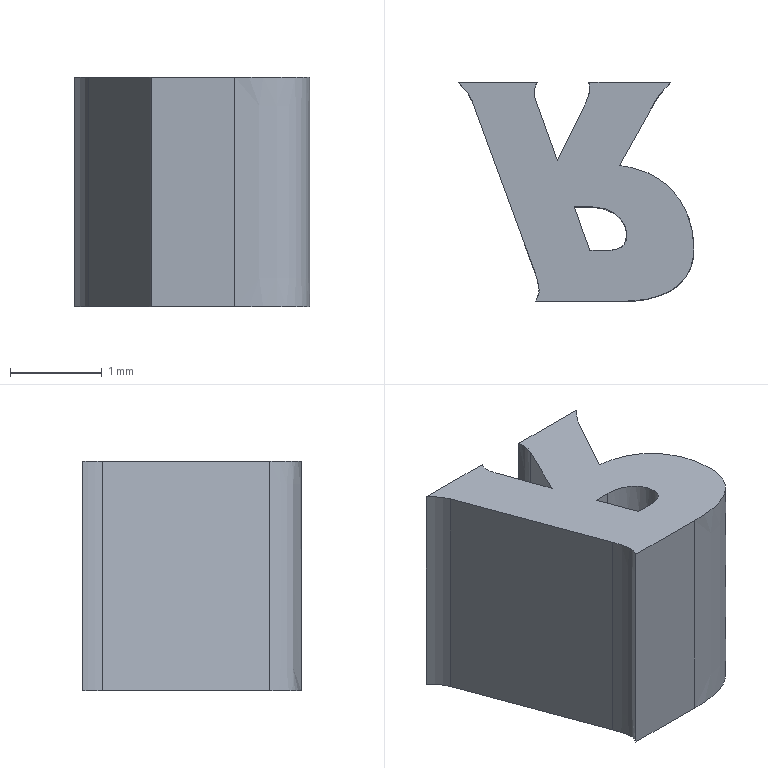Part | STEP file | lll_id1094_x_t | 1 solid | 23 faces | box 2.571 x 2.384 x 2.5 mm | volume 9.133 mm3 | plane 12 | other 6 | cylinder 5 | commonest cylinder face diameters 0.399 x1 1.039 x1 1.183 x1 1.552 x1 2.628 x1
STEP:
#1=CARTESIAN_POINT('',(386.73,-124.408,2.35));
#2=VERTEX_POINT('',#1);
#3=CARTESIAN_POINT('',(386.771,-124.406,2.35));
#4=VERTEX_POINT('',#3);
#5=CARTESIAN_POINT('',(386.726,-123.816,2.35));
#6=DIRECTION('',(0.,0.,1.));
#7=DIRECTION('',(0.,1.,0.));
#8=AXIS2_PLACEMENT_3D('',#5,#6,#7);
#9=CIRCLE('',#8,0.5916);
#10=EDGE_CURVE('',#2,#4,#9,.T.);
#11=ORIENTED_EDGE('',*,*,#10,.T.);
#12=CARTESIAN_POINT('',(386.771,-124.406,-0.15));
#13=VERTEX_POINT('',#12);
#14=CARTESIAN_POINT('',(386.771,-124.406,-0.15));
#15=DIRECTION('',(0.,0.,1.));
#16=VECTOR('',#15,1.);
#17=LINE('',#14,#16);
#18=EDGE_CURVE('',#13,#4,#17,.T.);
#19=ORIENTED_EDGE('',*,*,#18,.F.);
#20=CARTESIAN_POINT('',(386.73,-124.408,-0.15));
#21=VERTEX_POINT('',#20);
#22=CARTESIAN_POINT('',(386.726,-123.816,-0.15));
#23=DIRECTION('',(0.,0.,1.));
#24=DIRECTION('',(-1.,0.,0.));
#25=AXIS2_PLACEMENT_3D('',#22,#23,#24);
#26=CIRCLE('',#25,0.5916);
#27=EDGE_CURVE('',#21,#13,#26,.T.);
#28=ORIENTED_EDGE('',*,*,#27,.F.);
#29=CARTESIAN_POINT('',(386.73,-124.408,-0.15));
#30=DIRECTION('',(0.,0.,1.));
#31=VECTOR('',#30,1.);
#32=LINE('',#29,#31);
#33=EDGE_CURVE('',#21,#2,#32,.T.);
#34=ORIENTED_EDGE('',*,*,#33,.T.);
#35=EDGE_LOOP('',(#11,#19,#28,#34));
#36=FACE_OUTER_BOUND('',#35,.T.);
#37=CARTESIAN_POINT('',(386.726,-123.816,-0.15));
#38=DIRECTION('',(0.,0.,1.));
#39=DIRECTION('',(1.,0.,0.));
#40=AXIS2_PLACEMENT_3D('',#37,#38,#39);
#41=CYLINDRICAL_SURFACE('',#40,0.5916);
#42=ADVANCED_FACE('',(#36),#41,.F.);
#43=CARTESIAN_POINT('',(386.916,-124.343,2.35));
#44=VERTEX_POINT('',#43);
#45=CARTESIAN_POINT('',(386.771,-124.406,2.35));
#46=CARTESIAN_POINT('',(386.794,-124.405,2.35));
#47=CARTESIAN_POINT('',(386.816,-124.4,2.35));
#48=CARTESIAN_POINT('',(386.853,-124.389,2.35));
#49=CARTESIAN_POINT('',(386.867,-124.382,2.35));
#50=CARTESIAN_POINT('',(386.894,-124.366,2.35));
#51=CARTESIAN_POINT('',(386.906,-124.355,2.35));
#52=CARTESIAN_POINT('',(386.916,-124.343,2.35));
#53=(BOUNDED_CURVE()B_SPLINE_CURVE(3,(#45,#46,#47,#48,#49,#50,#51,#52),.UNSPECIFIED.,.F.,.F.)B_SPLINE_CURVE_WITH_KNOTS((4,2,2,4),(0.,0.418,0.7101,1.),.UNSPECIFIED.)CURVE()GEOMETRIC_REPRESENTATION_ITEM()RATIONAL_B_SPLINE_CURVE((0.5001,0.4979,0.4979,0.4976,0.4976,0.495,0.495,0.5001))REPRESENTATION_ITEM(''));
#54=EDGE_CURVE('',#4,#44,#53,.T.);
#55=ORIENTED_EDGE('',*,*,#54,.T.);
#56=CARTESIAN_POINT('',(386.916,-124.343,-0.15));
#57=VERTEX_POINT('',#56);
#58=CARTESIAN_POINT('',(386.916,-124.343,-0.15));
#59=DIRECTION('',(0.,0.,1.));
#60=VECTOR('',#59,1.);
#61=LINE('',#58,#60);
#62=EDGE_CURVE('',#57,#44,#61,.T.);
#63=ORIENTED_EDGE('',*,*,#62,.F.);
#64=CARTESIAN_POINT('',(386.771,-124.406,-0.15));
#65=CARTESIAN_POINT('',(386.794,-124.405,-0.15));
#66=CARTESIAN_POINT('',(386.816,-124.4,-0.15));
#67=CARTESIAN_POINT('',(386.853,-124.389,-0.15));
#68=CARTESIAN_POINT('',(386.867,-124.382,-0.15));
#69=CARTESIAN_POINT('',(386.894,-124.366,-0.15));
#70=CARTESIAN_POINT('',(386.906,-124.355,-0.15));
#71=CARTESIAN_POINT('',(386.916,-124.343,-0.15));
#72=(BOUNDED_CURVE()B_SPLINE_CURVE(3,(#64,#65,#66,#67,#68,#69,#70,#71),.UNSPECIFIED.,.F.,.F.)B_SPLINE_CURVE_WITH_KNOTS((4,2,2,4),(0.,0.418,0.7101,1.),.UNSPECIFIED.)CURVE()GEOMETRIC_REPRESENTATION_ITEM()RATIONAL_B_SPLINE_CURVE((0.5001,0.4979,0.4979,0.4976,0.4976,0.495,0.495,0.5001))REPRESENTATION_ITEM(''));
#73=EDGE_CURVE('',#13,#57,#72,.T.);
#74=ORIENTED_EDGE('',*,*,#73,.F.);
#75=ORIENTED_EDGE('',*,*,#18,.T.);
#76=EDGE_LOOP('',(#55,#63,#74,#75));
#77=FACE_OUTER_BOUND('',#76,.T.);
#78=CARTESIAN_POINT('',(386.771,-124.406,-0.15));
#79=CARTESIAN_POINT('',(386.794,-124.405,-0.15));
#80=CARTESIAN_POINT('',(386.816,-124.4,-0.15));
#81=CARTESIAN_POINT('',(386.853,-124.389,-0.15));
#82=CARTESIAN_POINT('',(386.867,-124.382,-0.15));
#83=CARTESIAN_POINT('',(386.894,-124.366,-0.15));
#84=CARTESIAN_POINT('',(386.906,-124.355,-0.15));
#85=CARTESIAN_POINT('',(386.916,-124.343,-0.15));
#86=(BOUNDED_CURVE()B_SPLINE_CURVE(3,(#78,#79,#80,#81,#82,#83,#84,#85),.UNSPECIFIED.,.F.,.F.)B_SPLINE_CURVE_WITH_KNOTS((4,2,2,4),(0.,0.418,0.7101,1.),.UNSPECIFIED.)CURVE()GEOMETRIC_REPRESENTATION_ITEM()RATIONAL_B_SPLINE_CURVE((0.5001,0.4979,0.4979,0.4976,0.4976,0.495,0.495,0.5001))REPRESENTATION_ITEM(''));
#87=DIRECTION('',(0.,0.,1.));
#88=VECTOR('',#87,1.);
#89=SURFACE_OF_LINEAR_EXTRUSION('',#86,#88);
#90=ADVANCED_FACE('',(#77),#89,.F.);
#91=CARTESIAN_POINT('',(386.549,-123.934,2.35));
#92=VERTEX_POINT('',#91);
#93=CARTESIAN_POINT('',(386.916,-124.343,2.35));
#94=CARTESIAN_POINT('',(386.927,-124.328,2.35));
#95=CARTESIAN_POINT('',(386.935,-124.312,2.35));
#96=CARTESIAN_POINT('',(386.942,-124.278,2.35));
#97=CARTESIAN_POINT('',(386.944,-124.263,2.35));
#98=CARTESIAN_POINT('',(386.943,-124.185,2.35));
#99=CARTESIAN_POINT('',(386.922,-124.126,2.35));
#100=CARTESIAN_POINT('',(386.859,-124.046,2.35));
#101=CARTESIAN_POINT('',(386.828,-124.018,2.35));
#102=CARTESIAN_POINT('',(386.759,-123.976,2.35));
#103=CARTESIAN_POINT('',(386.722,-123.96,2.35));
#104=CARTESIAN_POINT('',(386.656,-123.944,2.35));
#105=CARTESIAN_POINT('',(386.629,-123.939,2.35));
#106=CARTESIAN_POINT('',(386.589,-123.936,2.35));
#107=CARTESIAN_POINT('',(386.576,-123.935,2.35));
#108=CARTESIAN_POINT('',(386.558,-123.934,2.35));
#109=CARTESIAN_POINT('',(386.553,-123.934,2.35));
#110=CARTESIAN_POINT('',(386.549,-123.934,2.35));
#111=(BOUNDED_CURVE()B_SPLINE_CURVE(3,(#93,#94,#95,#96,#97,#98,#99,#100,#101,#102,#103,#104,#105,#106,#107,#108,#109,#110),.UNSPECIFIED.,.F.,.F.)B_SPLINE_CURVE_WITH_KNOTS((4,2,2,2,2,2,2,2,4),(0.,0.08567,0.1598,0.4394,0.6214,0.8013,0.9206,0.9801,1.),.UNSPECIFIED.)CURVE()GEOMETRIC_REPRESENTATION_ITEM()RATIONAL_B_SPLINE_CURVE((0.5001,0.4929,0.4929,0.4976,0.4976,0.4831,0.4831,0.4948,0.4948,0.4962,0.4962,0.4991,0.4991,0.5,0.5,0.5001,0.5001,0.5001))REPRESENTATION_ITEM(''));
#112=EDGE_CURVE('',#44,#92,#111,.T.);
#113=ORIENTED_EDGE('',*,*,#112,.T.);
#114=CARTESIAN_POINT('',(386.549,-123.934,-0.15));
#115=VERTEX_POINT('',#114);
#116=CARTESIAN_POINT('',(386.549,-123.934,-0.15));
#117=DIRECTION('',(0.,0.,1.));
#118=VECTOR('',#117,1.);
#119=LINE('',#116,#118);
#120=EDGE_CURVE('',#115,#92,#119,.T.);
#121=ORIENTED_EDGE('',*,*,#120,.F.);
#122=CARTESIAN_POINT('',(386.916,-124.343,-0.15));
#123=CARTESIAN_POINT('',(386.927,-124.328,-0.15));
#124=CARTESIAN_POINT('',(386.935,-124.312,-0.15));
#125=CARTESIAN_POINT('',(386.942,-124.278,-0.15));
#126=CARTESIAN_POINT('',(386.944,-124.263,-0.15));
#127=CARTESIAN_POINT('',(386.943,-124.185,-0.15));
#128=CARTESIAN_POINT('',(386.922,-124.126,-0.15));
#129=CARTESIAN_POINT('',(386.859,-124.046,-0.15));
#130=CARTESIAN_POINT('',(386.828,-124.018,-0.15));
#131=CARTESIAN_POINT('',(386.759,-123.976,-0.15));
#132=CARTESIAN_POINT('',(386.722,-123.96,-0.15));
#133=CARTESIAN_POINT('',(386.656,-123.944,-0.15));
#134=CARTESIAN_POINT('',(386.629,-123.939,-0.15));
#135=CARTESIAN_POINT('',(386.589,-123.936,-0.15));
#136=CARTESIAN_POINT('',(386.576,-123.935,-0.15));
#137=CARTESIAN_POINT('',(386.558,-123.934,-0.15));
#138=CARTESIAN_POINT('',(386.553,-123.934,-0.15));
#139=CARTESIAN_POINT('',(386.549,-123.934,-0.15));
#140=(BOUNDED_CURVE()B_SPLINE_CURVE(3,(#122,#123,#124,#125,#126,#127,#128,#129,#130,#131,#132,#133,#134,#135,#136,#137,#138,#139),.UNSPECIFIED.,.F.,.F.)B_SPLINE_CURVE_WITH_KNOTS((4,2,2,2,2,2,2,2,4),(0.,0.08567,0.1598,0.4394,0.6214,0.8013,0.9206,0.9801,1.),.UNSPECIFIED.)CURVE()GEOMETRIC_REPRESENTATION_ITEM()RATIONAL_B_SPLINE_CURVE((0.5001,0.4929,0.4929,0.4976,0.4976,0.4831,0.4831,0.4948,0.4948,0.4962,0.4962,0.4991,0.4991,0.5,0.5,0.5001,0.5001,0.5001))REPRESENTATION_ITEM(''));
#141=EDGE_CURVE('',#57,#115,#140,.T.);
#142=ORIENTED_EDGE('',*,*,#141,.F.);
#143=ORIENTED_EDGE('',*,*,#62,.T.);
#144=EDGE_LOOP('',(#113,#121,#142,#143));
#145=FACE_OUTER_BOUND('',#144,.T.);
#146=CARTESIAN_POINT('',(386.916,-124.343,-0.15));
#147=CARTESIAN_POINT('',(386.927,-124.328,-0.15));
#148=CARTESIAN_POINT('',(386.935,-124.312,-0.15));
#149=CARTESIAN_POINT('',(386.942,-124.278,-0.15));
#150=CARTESIAN_POINT('',(386.944,-124.263,-0.15));
#151=CARTESIAN_POINT('',(386.943,-124.185,-0.15));
#152=CARTESIAN_POINT('',(386.922,-124.126,-0.15));
#153=CARTESIAN_POINT('',(386.859,-124.046,-0.15));
#154=CARTESIAN_POINT('',(386.828,-124.018,-0.15));
#155=CARTESIAN_POINT('',(386.759,-123.976,-0.15));
#156=CARTESIAN_POINT('',(386.722,-123.96,-0.15));
#157=CARTESIAN_POINT('',(386.656,-123.944,-0.15));
#158=CARTESIAN_POINT('',(386.629,-123.939,-0.15));
#159=CARTESIAN_POINT('',(386.589,-123.936,-0.15));
#160=CARTESIAN_POINT('',(386.576,-123.935,-0.15));
#161=CARTESIAN_POINT('',(386.558,-123.934,-0.15));
#162=CARTESIAN_POINT('',(386.553,-123.934,-0.15));
#163=CARTESIAN_POINT('',(386.549,-123.934,-0.15));
#164=(BOUNDED_CURVE()B_SPLINE_CURVE(3,(#146,#147,#148,#149,#150,#151,#152,#153,#154,#155,#156,#157,#158,#159,#160,#161,#162,#163),.UNSPECIFIED.,.F.,.F.)B_SPLINE_CURVE_WITH_KNOTS((4,2,2,2,2,2,2,2,4),(0.,0.08567,0.1598,0.4394,0.6214,0.8013,0.9206,0.9801,1.),.UNSPECIFIED.)CURVE()GEOMETRIC_REPRESENTATION_ITEM()RATIONAL_B_SPLINE_CURVE((0.5001,0.4929,0.4929,0.4976,0.4976,0.4831,0.4831,0.4948,0.4948,0.4962,0.4962,0.4991,0.4991,0.5,0.5,0.5001,0.5001,0.5001))REPRESENTATION_ITEM(''));
#165=DIRECTION('',(0.,0.,1.));
#166=VECTOR('',#165,1.);
#167=SURFACE_OF_LINEAR_EXTRUSION('',#164,#166);
#168=ADVANCED_FACE('',(#145),#167,.F.);
#169=CARTESIAN_POINT('',(386.37,-123.934,2.35));
#170=VERTEX_POINT('',#169);
#171=CARTESIAN_POINT('',(386.549,-123.934,2.35));
#172=DIRECTION('',(-1.,0.,0.));
#173=VECTOR('',#172,1.);
#174=LINE('',#171,#173);
#175=EDGE_CURVE('',#92,#170,#174,.T.);
#176=ORIENTED_EDGE('',*,*,#175,.T.);
#177=CARTESIAN_POINT('',(386.37,-123.934,-0.15));
#178=VERTEX_POINT('',#177);
#179=CARTESIAN_POINT('',(386.37,-123.934,-0.15));
#180=DIRECTION('',(0.,0.,1.));
#181=VECTOR('',#180,1.);
#182=LINE('',#179,#181);
#183=EDGE_CURVE('',#178,#170,#182,.T.);
#184=ORIENTED_EDGE('',*,*,#183,.F.);
#185=CARTESIAN_POINT('',(386.549,-123.934,-0.15));
#186=DIRECTION('',(-1.,0.,0.));
#187=VECTOR('',#186,1.);
#188=LINE('',#185,#187);
#189=EDGE_CURVE('',#115,#178,#188,.T.);
#190=ORIENTED_EDGE('',*,*,#189,.F.);
#191=ORIENTED_EDGE('',*,*,#120,.T.);
#192=EDGE_LOOP('',(#176,#184,#190,#191));
#193=FACE_OUTER_BOUND('',#192,.T.);
#194=CARTESIAN_POINT('',(386.549,-123.934,-0.15));
#195=DIRECTION('',(0.,1.,0.));
#196=DIRECTION('',(0.,0.,1.));
#197=AXIS2_PLACEMENT_3D('',#194,#195,#196);
#198=PLANE('',#197);
#199=ADVANCED_FACE('',(#193),#198,.F.);
#200=CARTESIAN_POINT('',(386.543,-124.408,2.35));
#201=VERTEX_POINT('',#200);
#202=CARTESIAN_POINT('',(386.37,-123.934,2.35));
#203=DIRECTION('',(0.3422,-0.9396,0.));
#204=VECTOR('',#203,1.);
#205=LINE('',#202,#204);
#206=EDGE_CURVE('',#170,#201,#205,.T.);
#207=ORIENTED_EDGE('',*,*,#206,.T.);
#208=CARTESIAN_POINT('',(386.543,-124.408,-0.15));
#209=VERTEX_POINT('',#208);
#210=CARTESIAN_POINT('',(386.543,-124.408,-0.15));
#211=DIRECTION('',(0.,0.,1.));
#212=VECTOR('',#211,1.);
#213=LINE('',#210,#212);
#214=EDGE_CURVE('',#209,#201,#213,.T.);
#215=ORIENTED_EDGE('',*,*,#214,.F.);
#216=CARTESIAN_POINT('',(386.37,-123.934,-0.15));
#217=DIRECTION('',(0.3422,-0.9396,0.));
#218=VECTOR('',#217,1.);
#219=LINE('',#216,#218);
#220=EDGE_CURVE('',#178,#209,#219,.T.);
#221=ORIENTED_EDGE('',*,*,#220,.F.);
#222=ORIENTED_EDGE('',*,*,#183,.T.);
#223=EDGE_LOOP('',(#207,#215,#221,#222));
#224=FACE_OUTER_BOUND('',#223,.T.);
#225=CARTESIAN_POINT('',(386.37,-123.934,-0.15));
#226=DIRECTION('',(-0.9396,-0.3422,0.));
#227=DIRECTION('',(-0.3422,0.9396,0.));
#228=AXIS2_PLACEMENT_3D('',#225,#226,#227);
#229=PLANE('',#228);
#230=ADVANCED_FACE('',(#224),#229,.F.);
#231=CARTESIAN_POINT('',(387.422,-122.581,2.35));
#232=VERTEX_POINT('',#231);
#233=CARTESIAN_POINT('',(387.25,-122.793,2.35));
#234=VERTEX_POINT('',#233);
#235=CARTESIAN_POINT('',(387.925,-123.174,2.35));
#236=DIRECTION('',(0.,0.,1.));
#237=DIRECTION('',(-1.,0.,0.));
#238=AXIS2_PLACEMENT_3D('',#235,#236,#237);
#239=CIRCLE('',#238,0.7758);
#240=EDGE_CURVE('',#232,#234,#239,.T.);
#241=ORIENTED_EDGE('',*,*,#240,.T.);
#242=CARTESIAN_POINT('',(387.25,-122.793,-0.15));
#243=VERTEX_POINT('',#242);
#244=CARTESIAN_POINT('',(387.25,-122.793,-0.15));
#245=DIRECTION('',(0.,0.,1.));
#246=VECTOR('',#245,1.);
#247=LINE('',#244,#246);
#248=EDGE_CURVE('',#243,#234,#247,.T.);
#249=ORIENTED_EDGE('',*,*,#248,.F.);
#250=CARTESIAN_POINT('',(387.422,-122.581,-0.15));
#251=VERTEX_POINT('',#250);
#252=CARTESIAN_POINT('',(387.925,-123.174,-0.15));
#253=DIRECTION('',(0.,0.,1.));
#254=DIRECTION('',(-1.,0.,0.));
#255=AXIS2_PLACEMENT_3D('',#252,#253,#254);
#256=CIRCLE('',#255,0.7758);
#257=EDGE_CURVE('',#251,#243,#256,.T.);
#258=ORIENTED_EDGE('',*,*,#257,.F.);
#259=CARTESIAN_POINT('',(387.429,-122.578,-0.15));
#260=DIRECTION('',(0.,0.,1.));
#261=VECTOR('',#260,1.);
#262=LINE('',#259,#261);
#263=EDGE_CURVE('',#251,#232,#262,.T.);
#264=ORIENTED_EDGE('',*,*,#263,.T.);
#265=EDGE_LOOP('',(#241,#249,#258,#264));
#266=FACE_OUTER_BOUND('',#265,.T.);
#267=CARTESIAN_POINT('',(387.925,-123.174,-0.15));
#268=DIRECTION('',(0.,0.,1.));
#269=DIRECTION('',(1.,0.,0.));
#270=AXIS2_PLACEMENT_3D('',#267,#268,#269);
#271=CYLINDRICAL_SURFACE('',#270,0.7758);
#272=ADVANCED_FACE('',(#266),#271,.F.);
#273=CARTESIAN_POINT('',(386.864,-123.485,2.35));
#274=VERTEX_POINT('',#273);
#275=CARTESIAN_POINT('',(387.25,-122.793,2.35));
#276=DIRECTION('',(-0.4865,-0.8737,0.));
#277=VECTOR('',#276,1.);
#278=LINE('',#275,#277);
#279=EDGE_CURVE('',#234,#274,#278,.T.);
#280=ORIENTED_EDGE('',*,*,#279,.T.);
#281=CARTESIAN_POINT('',(386.864,-123.485,-0.15));
#282=VERTEX_POINT('',#281);
#283=CARTESIAN_POINT('',(386.864,-123.485,-0.15));
#284=DIRECTION('',(0.,0.,1.));
#285=VECTOR('',#284,1.);
#286=LINE('',#283,#285);
#287=EDGE_CURVE('',#282,#274,#286,.T.);
#288=ORIENTED_EDGE('',*,*,#287,.F.);
#289=CARTESIAN_POINT('',(387.25,-122.793,-0.15));
#290=DIRECTION('',(-0.4865,-0.8737,0.));
#291=VECTOR('',#290,1.);
#292=LINE('',#289,#291);
#293=EDGE_CURVE('',#243,#282,#292,.T.);
#294=ORIENTED_EDGE('',*,*,#293,.F.);
#295=ORIENTED_EDGE('',*,*,#248,.T.);
#296=EDGE_LOOP('',(#280,#288,#294,#295));
#297=FACE_OUTER_BOUND('',#296,.T.);
#298=CARTESIAN_POINT('',(387.25,-122.793,-0.15));
#299=DIRECTION('',(-0.8737,0.4865,0.));
#300=DIRECTION('',(0.4865,0.8737,0.));
#301=AXIS2_PLACEMENT_3D('',#298,#299,#300);
#302=PLANE('',#301);
#303=ADVANCED_FACE('',(#297),#302,.F.);
#304=CARTESIAN_POINT('',(387.016,-123.513,2.35));
#305=VERTEX_POINT('',#304);
#306=CARTESIAN_POINT('',(386.706,-124.79,2.35));
#307=DIRECTION('',(0.,0.,-1.));
#308=DIRECTION('',(0.,-1.,0.));
#309=AXIS2_PLACEMENT_3D('',#306,#307,#308);
#310=CIRCLE('',#309,1.314);
#311=EDGE_CURVE('',#274,#305,#310,.T.);
#312=ORIENTED_EDGE('',*,*,#311,.T.);
#313=CARTESIAN_POINT('',(387.016,-123.513,-0.15));
#314=VERTEX_POINT('',#313);
#315=CARTESIAN_POINT('',(387.016,-123.513,-0.15));
#316=DIRECTION('',(0.,0.,1.));
#317=VECTOR('',#316,1.);
#318=LINE('',#315,#317);
#319=EDGE_CURVE('',#314,#305,#318,.T.);
#320=ORIENTED_EDGE('',*,*,#319,.F.);
#321=CARTESIAN_POINT('',(386.706,-124.79,-0.15));
#322=DIRECTION('',(0.,0.,-1.));
#323=DIRECTION('',(1.,0.,0.));
#324=AXIS2_PLACEMENT_3D('',#321,#322,#323);
#325=CIRCLE('',#324,1.314);
#326=EDGE_CURVE('',#282,#314,#325,.T.);
#327=ORIENTED_EDGE('',*,*,#326,.F.);
#328=ORIENTED_EDGE('',*,*,#287,.T.);
#329=EDGE_LOOP('',(#312,#320,#327,#328));
#330=FACE_OUTER_BOUND('',#329,.T.);
#331=CARTESIAN_POINT('',(386.706,-124.79,-0.15));
#332=DIRECTION('',(0.,0.,1.));
#333=DIRECTION('',(1.,0.,0.));
#334=AXIS2_PLACEMENT_3D('',#331,#332,#333);
#335=CYLINDRICAL_SURFACE('',#334,1.314);
#336=ADVANCED_FACE('',(#330),#335,.T.);
#337=CARTESIAN_POINT('',(386.856,-124.962,2.35));
#338=VERTEX_POINT('',#337);
#339=CARTESIAN_POINT('',(387.016,-123.513,2.35));
#340=CARTESIAN_POINT('',(387.307,-123.577,2.35));
#341=CARTESIAN_POINT('',(387.527,-123.776,2.35));
#342=CARTESIAN_POINT('',(387.656,-124.17,2.35));
#343=CARTESIAN_POINT('',(387.674,-124.285,2.35));
#344=CARTESIAN_POINT('',(387.673,-124.447,2.35));
#345=CARTESIAN_POINT('',(387.667,-124.492,2.35));
#346=CARTESIAN_POINT('',(387.628,-124.658,2.35));
#347=CARTESIAN_POINT('',(387.555,-124.761,2.35));
#348=CARTESIAN_POINT('',(387.406,-124.858,2.35));
#349=CARTESIAN_POINT('',(387.359,-124.88,2.35));
#350=CARTESIAN_POINT('',(387.25,-124.918,2.35));
#351=CARTESIAN_POINT('',(387.188,-124.934,2.35));
#352=CARTESIAN_POINT('',(387.061,-124.954,2.35));
#353=CARTESIAN_POINT('',(386.997,-124.96,2.35));
#354=CARTESIAN_POINT('',(386.907,-124.962,2.35));
#355=CARTESIAN_POINT('',(386.881,-124.962,2.35));
#356=CARTESIAN_POINT('',(386.856,-124.962,2.35));
#357=(BOUNDED_CURVE()B_SPLINE_CURVE(3,(#339,#340,#341,#342,#343,#344,#345,#346,#347,#348,#349,#350,#351,#352,#353,#354,#355,#356),.UNSPECIFIED.,.F.,.F.)B_SPLINE_CURVE_WITH_KNOTS((4,2,2,2,2,2,2,2,4),(0.,0.3873,0.5378,0.596,0.7502,0.8132,0.891,0.969,1.),.UNSPECIFIED.)CURVE()GEOMETRIC_REPRESENTATION_ITEM()RATIONAL_B_SPLINE_CURVE((0.5004,0.4564,0.4564,0.496,0.496,0.4986,0.4986,0.4762,0.4762,0.498,0.498,0.499,0.499,0.4997,0.4997,0.5004,0.5004,0.5004))REPRESENTATION_ITEM(''));
#358=EDGE_CURVE('',#305,#338,#357,.T.);
#359=ORIENTED_EDGE('',*,*,#358,.T.);
#360=CARTESIAN_POINT('',(386.856,-124.962,-0.15));
#361=VERTEX_POINT('',#360);
#362=CARTESIAN_POINT('',(386.856,-124.962,-0.15));
#363=DIRECTION('',(0.,0.,1.));
#364=VECTOR('',#363,1.);
#365=LINE('',#362,#364);
#366=EDGE_CURVE('',#361,#338,#365,.T.);
#367=ORIENTED_EDGE('',*,*,#366,.F.);
#368=CARTESIAN_POINT('',(387.016,-123.513,-0.15));
#369=CARTESIAN_POINT('',(387.307,-123.577,-0.15));
#370=CARTESIAN_POINT('',(387.527,-123.776,-0.15));
#371=CARTESIAN_POINT('',(387.656,-124.17,-0.15));
#372=CARTESIAN_POINT('',(387.674,-124.285,-0.15));
#373=CARTESIAN_POINT('',(387.673,-124.447,-0.15));
#374=CARTESIAN_POINT('',(387.667,-124.492,-0.15));
#375=CARTESIAN_POINT('',(387.628,-124.658,-0.15));
#376=CARTESIAN_POINT('',(387.555,-124.761,-0.15));
#377=CARTESIAN_POINT('',(387.406,-124.858,-0.15));
#378=CARTESIAN_POINT('',(387.359,-124.88,-0.15));
#379=CARTESIAN_POINT('',(387.25,-124.918,-0.15));
#380=CARTESIAN_POINT('',(387.188,-124.934,-0.15));
#381=CARTESIAN_POINT('',(387.061,-124.954,-0.15));
#382=CARTESIAN_POINT('',(386.997,-124.96,-0.15));
#383=CARTESIAN_POINT('',(386.907,-124.962,-0.15));
#384=CARTESIAN_POINT('',(386.881,-124.962,-0.15));
#385=CARTESIAN_POINT('',(386.856,-124.962,-0.15));
#386=(BOUNDED_CURVE()B_SPLINE_CURVE(3,(#368,#369,#370,#371,#372,#373,#374,#375,#376,#377,#378,#379,#380,#381,#382,#383,#384,#385),.UNSPECIFIED.,.F.,.F.)B_SPLINE_CURVE_WITH_KNOTS((4,2,2,2,2,2,2,2,4),(0.,0.3873,0.5378,0.596,0.7502,0.8132,0.891,0.969,1.),.UNSPECIFIED.)CURVE()GEOMETRIC_REPRESENTATION_ITEM()RATIONAL_B_SPLINE_CURVE((0.5004,0.4564,0.4564,0.496,0.496,0.4986,0.4986,0.4762,0.4762,0.498,0.498,0.499,0.499,0.4997,0.4997,0.5004,0.5004,0.5004))REPRESENTATION_ITEM(''));
#387=EDGE_CURVE('',#314,#361,#386,.T.);
#388=ORIENTED_EDGE('',*,*,#387,.F.);
#389=ORIENTED_EDGE('',*,*,#319,.T.);
#390=EDGE_LOOP('',(#359,#367,#388,#389));
#391=FACE_OUTER_BOUND('',#390,.T.);
#392=CARTESIAN_POINT('',(387.016,-123.513,-0.15));
#393=CARTESIAN_POINT('',(387.307,-123.577,-0.15));
#394=CARTESIAN_POINT('',(387.527,-123.776,-0.15));
#395=CARTESIAN_POINT('',(387.656,-124.17,-0.15));
#396=CARTESIAN_POINT('',(387.674,-124.285,-0.15));
#397=CARTESIAN_POINT('',(387.673,-124.447,-0.15));
#398=CARTESIAN_POINT('',(387.667,-124.492,-0.15));
#399=CARTESIAN_POINT('',(387.628,-124.658,-0.15));
#400=CARTESIAN_POINT('',(387.555,-124.761,-0.15));
#401=CARTESIAN_POINT('',(387.406,-124.858,-0.15));
#402=CARTESIAN_POINT('',(387.359,-124.88,-0.15));
#403=CARTESIAN_POINT('',(387.25,-124.918,-0.15));
#404=CARTESIAN_POINT('',(387.188,-124.934,-0.15));
#405=CARTESIAN_POINT('',(387.061,-124.954,-0.15));
#406=CARTESIAN_POINT('',(386.997,-124.96,-0.15));
#407=CARTESIAN_POINT('',(386.907,-124.962,-0.15));
#408=CARTESIAN_POINT('',(386.881,-124.962,-0.15));
#409=CARTESIAN_POINT('',(386.856,-124.962,-0.15));
#410=(BOUNDED_CURVE()B_SPLINE_CURVE(3,(#392,#393,#394,#395,#396,#397,#398,#399,#400,#401,#402,#403,#404,#405,#406,#407,#408,#409),.UNSPECIFIED.,.F.,.F.)B_SPLINE_CURVE_WITH_KNOTS((4,2,2,2,2,2,2,2,4),(0.,0.3873,0.5378,0.596,0.7502,0.8132,0.891,0.969,1.),.UNSPECIFIED.)CURVE()GEOMETRIC_REPRESENTATION_ITEM()RATIONAL_B_SPLINE_CURVE((0.5004,0.4564,0.4564,0.496,0.496,0.4986,0.4986,0.4762,0.4762,0.498,0.498,0.499,0.499,0.4997,0.4997,0.5004,0.5004,0.5004))REPRESENTATION_ITEM(''));
#411=DIRECTION('',(0.,0.,1.));
#412=VECTOR('',#411,1.);
#413=SURFACE_OF_LINEAR_EXTRUSION('',#410,#412);
#414=ADVANCED_FACE('',(#391),#413,.F.);
#415=CARTESIAN_POINT('',(385.951,-124.959,2.35));
#416=VERTEX_POINT('',#415);
#417=CARTESIAN_POINT('',(386.856,-124.962,2.35));
#418=DIRECTION('',(-1.,0.,0.));
#419=VECTOR('',#418,1.);
#420=LINE('',#417,#419);
#421=EDGE_CURVE('',#338,#416,#420,.T.);
#422=ORIENTED_EDGE('',*,*,#421,.T.);
#423=CARTESIAN_POINT('',(385.951,-124.959,-0.15));
#424=VERTEX_POINT('',#423);
#425=CARTESIAN_POINT('',(385.946,-124.962,-0.15));
#426=DIRECTION('',(0.,0.,1.));
#427=VECTOR('',#426,1.);
#428=LINE('',#425,#427);
#429=EDGE_CURVE('',#424,#416,#428,.T.);
#430=ORIENTED_EDGE('',*,*,#429,.F.);
#431=CARTESIAN_POINT('',(386.856,-124.962,-0.15));
#432=DIRECTION('',(-1.,0.,0.));
#433=VECTOR('',#432,1.);
#434=LINE('',#431,#433);
#435=EDGE_CURVE('',#361,#424,#434,.T.);
#436=ORIENTED_EDGE('',*,*,#435,.F.);
#437=ORIENTED_EDGE('',*,*,#366,.T.);
#438=EDGE_LOOP('',(#422,#430,#436,#437));
#439=FACE_OUTER_BOUND('',#438,.T.);
#440=CARTESIAN_POINT('',(386.856,-124.962,-0.15));
#441=DIRECTION('',(0.,1.,0.));
#442=DIRECTION('',(0.,0.,1.));
#443=AXIS2_PLACEMENT_3D('',#440,#441,#442);
#444=PLANE('',#443);
#445=ADVANCED_FACE('',(#439),#444,.F.);
#446=CARTESIAN_POINT('',(385.934,-124.618,2.35));
#447=VERTEX_POINT('',#446);
#448=CARTESIAN_POINT('',(385.951,-124.956,2.35));
#449=CARTESIAN_POINT('',(385.953,-124.954,2.35));
#450=CARTESIAN_POINT('',(385.956,-124.951,2.35));
#451=CARTESIAN_POINT('',(385.975,-124.925,2.35));
#452=CARTESIAN_POINT('',(385.985,-124.899,2.35));
#453=CARTESIAN_POINT('',(385.99,-124.858,2.35));
#454=CARTESIAN_POINT('',(385.991,-124.845,2.35));
#455=CARTESIAN_POINT('',(385.989,-124.821,2.35));
#456=CARTESIAN_POINT('',(385.988,-124.81,2.35));
#457=CARTESIAN_POINT('',(385.984,-124.789,2.35));
#458=CARTESIAN_POINT('',(385.982,-124.778,2.35));
#459=CARTESIAN_POINT('',(385.977,-124.756,2.35));
#460=CARTESIAN_POINT('',(385.974,-124.745,2.35));
#461=CARTESIAN_POINT('',(385.964,-124.71,2.35));
#462=CARTESIAN_POINT('',(385.957,-124.685,2.35));
#463=CARTESIAN_POINT('',(385.944,-124.646,2.35));
#464=CARTESIAN_POINT('',(385.939,-124.632,2.35));
#465=CARTESIAN_POINT('',(385.934,-124.618,2.35));
#466=(BOUNDED_CURVE()B_SPLINE_CURVE(3,(#448,#449,#450,#451,#452,#453,#454,#455,#456,#457,#458,#459,#460,#461,#462,#463,#464,#465),.UNSPECIFIED.,.F.,.F.)B_SPLINE_CURVE_WITH_KNOTS((4,2,2,2,2,2,2,2,4),(0.,0.03213,0.269,0.3783,0.4714,0.5647,0.6581,0.8757,1.),.UNSPECIFIED.)CURVE()GEOMETRIC_REPRESENTATION_ITEM()RATIONAL_B_SPLINE_CURVE((0.5001,0.5,0.5,0.4887,0.4887,0.4987,0.4987,0.4996,0.4996,0.4998,0.4998,0.5,0.5,0.5,0.5,0.5,0.5,0.5001))REPRESENTATION_ITEM(''));
#467=EDGE_CURVE('',#416,#447,#466,.T.);
#468=ORIENTED_EDGE('',*,*,#467,.T.);
#469=CARTESIAN_POINT('',(385.934,-124.618,-0.15));
#470=VERTEX_POINT('',#469);
#471=CARTESIAN_POINT('',(385.934,-124.618,-0.15));
#472=DIRECTION('',(0.,0.,1.));
#473=VECTOR('',#472,1.);
#474=LINE('',#471,#473);
#475=EDGE_CURVE('',#470,#447,#474,.T.);
#476=ORIENTED_EDGE('',*,*,#475,.F.);
#477=CARTESIAN_POINT('',(385.949,-124.959,-0.15));
#478=CARTESIAN_POINT('',(385.949,-124.958,-0.15));
#479=CARTESIAN_POINT('',(385.95,-124.957,-0.15));
#480=CARTESIAN_POINT('',(385.953,-124.954,-0.15));
#481=CARTESIAN_POINT('',(385.956,-124.951,-0.15));
#482=CARTESIAN_POINT('',(385.975,-124.925,-0.15));
#483=CARTESIAN_POINT('',(385.985,-124.899,-0.15));
#484=CARTESIAN_POINT('',(385.99,-124.858,-0.15));
#485=CARTESIAN_POINT('',(385.991,-124.845,-0.15));
#486=CARTESIAN_POINT('',(385.989,-124.821,-0.15));
#487=CARTESIAN_POINT('',(385.988,-124.81,-0.15));
#488=CARTESIAN_POINT('',(385.984,-124.789,-0.15));
#489=CARTESIAN_POINT('',(385.982,-124.778,-0.15));
#490=CARTESIAN_POINT('',(385.977,-124.756,-0.15));
#491=CARTESIAN_POINT('',(385.974,-124.745,-0.15));
#492=CARTESIAN_POINT('',(385.964,-124.71,-0.15));
#493=CARTESIAN_POINT('',(385.957,-124.685,-0.15));
#494=CARTESIAN_POINT('',(385.944,-124.646,-0.15));
#495=CARTESIAN_POINT('',(385.939,-124.632,-0.15));
#496=CARTESIAN_POINT('',(385.934,-124.618,-0.15));
#497=(BOUNDED_CURVE()B_SPLINE_CURVE(3,(#477,#478,#479,#480,#481,#482,#483,#484,#485,#486,#487,#488,#489,#490,#491,#492,#493,#494,#495,#496),.UNSPECIFIED.,.F.,.F.)B_SPLINE_CURVE_WITH_KNOTS((4,2,2,2,2,2,2,2,2,4),(0.,0.009901,0.04172,0.2762,0.3844,0.4766,0.569,0.6615,0.8769,1.),.UNSPECIFIED.)CURVE()GEOMETRIC_REPRESENTATION_ITEM()RATIONAL_B_SPLINE_CURVE((0.5001,0.5001,0.5001,0.5,0.5,0.4887,0.4887,0.4987,0.4987,0.4996,0.4996,0.4998,0.4998,0.5,0.5,0.5,0.5,0.5,0.5,0.5001))REPRESENTATION_ITEM(''));
#498=EDGE_CURVE('',#424,#470,#497,.T.);
#499=ORIENTED_EDGE('',*,*,#498,.F.);
#500=ORIENTED_EDGE('',*,*,#429,.T.);
#501=EDGE_LOOP('',(#468,#476,#499,#500));
#502=FACE_OUTER_BOUND('',#501,.T.);
#503=CARTESIAN_POINT('',(385.946,-124.962,-0.15));
#504=CARTESIAN_POINT('',(385.947,-124.961,-0.15));
#505=CARTESIAN_POINT('',(385.948,-124.96,-0.15));
#506=CARTESIAN_POINT('',(385.949,-124.958,-0.15));
#507=CARTESIAN_POINT('',(385.95,-124.957,-0.15));
#508=CARTESIAN_POINT('',(385.953,-124.954,-0.15));
#509=CARTESIAN_POINT('',(385.956,-124.951,-0.15));
#510=CARTESIAN_POINT('',(385.975,-124.925,-0.15));
#511=CARTESIAN_POINT('',(385.985,-124.899,-0.15));
#512=CARTESIAN_POINT('',(385.99,-124.858,-0.15));
#513=CARTESIAN_POINT('',(385.991,-124.845,-0.15));
#514=CARTESIAN_POINT('',(385.989,-124.821,-0.15));
#515=CARTESIAN_POINT('',(385.988,-124.81,-0.15));
#516=CARTESIAN_POINT('',(385.984,-124.789,-0.15));
#517=CARTESIAN_POINT('',(385.982,-124.778,-0.15));
#518=CARTESIAN_POINT('',(385.977,-124.756,-0.15));
#519=CARTESIAN_POINT('',(385.974,-124.745,-0.15));
#520=CARTESIAN_POINT('',(385.964,-124.71,-0.15));
#521=CARTESIAN_POINT('',(385.957,-124.685,-0.15));
#522=CARTESIAN_POINT('',(385.944,-124.646,-0.15));
#523=CARTESIAN_POINT('',(385.939,-124.632,-0.15));
#524=CARTESIAN_POINT('',(385.934,-124.618,-0.15));
#525=(BOUNDED_CURVE()B_SPLINE_CURVE(3,(#503,#504,#505,#506,#507,#508,#509,#510,#511,#512,#513,#514,#515,#516,#517,#518,#519,#520,#521,#522,#523,#524),.UNSPECIFIED.,.F.,.F.)B_SPLINE_CURVE_WITH_KNOTS((4,2,2,2,2,2,2,2,2,2,4),(0.,0.01012,0.01992,0.05142,0.2835,0.3906,0.4819,0.5734,0.665,0.8781,1.),.UNSPECIFIED.)CURVE()GEOMETRIC_REPRESENTATION_ITEM()RATIONAL_B_SPLINE_CURVE((0.5001,0.5001,0.5001,0.5001,0.5001,0.5,0.5,0.4887,0.4887,0.4987,0.4987,0.4996,0.4996,0.4998,0.4998,0.5,0.5,0.5,0.5,0.5,0.5,0.5001))REPRESENTATION_ITEM(''));
#526=DIRECTION('',(0.,0.,1.));
#527=VECTOR('',#526,1.);
#528=SURFACE_OF_LINEAR_EXTRUSION('',#525,#527);
#529=ADVANCED_FACE('',(#502),#528,.F.);
#530=CARTESIAN_POINT('',(385.265,-122.793,2.35));
#531=VERTEX_POINT('',#530);
#532=CARTESIAN_POINT('',(385.934,-124.618,2.35));
#533=DIRECTION('',(-0.3441,0.9389,0.));
#534=VECTOR('',#533,1.);
#535=LINE('',#532,#534);
#536=EDGE_CURVE('',#447,#531,#535,.T.);
#537=ORIENTED_EDGE('',*,*,#536,.T.);
#538=CARTESIAN_POINT('',(385.265,-122.793,-0.15));
#539=VERTEX_POINT('',#538);
#540=CARTESIAN_POINT('',(385.265,-122.793,-0.15));
#541=DIRECTION('',(0.,0.,1.));
#542=VECTOR('',#541,1.);
#543=LINE('',#540,#542);
#544=EDGE_CURVE('',#539,#531,#543,.T.);
#545=ORIENTED_EDGE('',*,*,#544,.F.);
#546=CARTESIAN_POINT('',(385.934,-124.618,-0.15));
#547=DIRECTION('',(-0.3441,0.9389,0.));
#548=VECTOR('',#547,1.);
#549=LINE('',#546,#548);
#550=EDGE_CURVE('',#470,#539,#549,.T.);
#551=ORIENTED_EDGE('',*,*,#550,.F.);
#552=ORIENTED_EDGE('',*,*,#475,.T.);
#553=EDGE_LOOP('',(#537,#545,#551,#552));
#554=FACE_OUTER_BOUND('',#553,.T.);
#555=CARTESIAN_POINT('',(385.934,-124.618,-0.15));
#556=DIRECTION('',(0.9389,0.3441,0.));
#557=DIRECTION('',(0.3441,-0.9389,0.));
#558=AXIS2_PLACEMENT_3D('',#555,#556,#557);
#559=PLANE('',#558);
#560=ADVANCED_FACE('',(#554),#559,.F.);
#561=CARTESIAN_POINT('',(385.108,-122.58,2.35));
#562=VERTEX_POINT('',#561);
#563=CARTESIAN_POINT('',(384.783,-122.988,2.35));
#564=DIRECTION('',(0.,0.,1.));
#565=DIRECTION('',(-1.,0.,0.));
#566=AXIS2_PLACEMENT_3D('',#563,#564,#565);
#567=CIRCLE('',#566,0.5196);
#568=EDGE_CURVE('',#531,#562,#567,.T.);
#569=ORIENTED_EDGE('',*,*,#568,.T.);
#570=CARTESIAN_POINT('',(385.108,-122.58,-0.15));
#571=VERTEX_POINT('',#570);
#572=CARTESIAN_POINT('',(385.102,-122.578,-0.15));
#573=DIRECTION('',(0.,0.,1.));
#574=VECTOR('',#573,1.);
#575=LINE('',#572,#574);
#576=EDGE_CURVE('',#571,#562,#575,.T.);
#577=ORIENTED_EDGE('',*,*,#576,.F.);
#578=CARTESIAN_POINT('',(384.783,-122.988,-0.15));
#579=DIRECTION('',(0.,0.,1.));
#580=DIRECTION('',(-1.,0.,0.));
#581=AXIS2_PLACEMENT_3D('',#578,#579,#580);
#582=CIRCLE('',#581,0.5196);
#583=EDGE_CURVE('',#539,#571,#582,.T.);
#584=ORIENTED_EDGE('',*,*,#583,.F.);
#585=ORIENTED_EDGE('',*,*,#544,.T.);
#586=EDGE_LOOP('',(#569,#577,#584,#585));
#587=FACE_OUTER_BOUND('',#586,.T.);
#588=CARTESIAN_POINT('',(384.783,-122.988,-0.15));
#589=DIRECTION('',(0.,0.,1.));
#590=DIRECTION('',(1.,0.,0.));
#591=AXIS2_PLACEMENT_3D('',#588,#589,#590);
#592=CYLINDRICAL_SURFACE('',#591,0.5196);
#593=ADVANCED_FACE('',(#587),#592,.F.);
#594=CARTESIAN_POINT('',(385.968,-122.58,2.35));
#595=VERTEX_POINT('',#594);
#596=CARTESIAN_POINT('',(385.108,-122.578,2.35));
#597=DIRECTION('',(1.,0.,0.));
#598=VECTOR('',#597,1.);
#599=LINE('',#596,#598);
#600=EDGE_CURVE('',#562,#595,#599,.T.);
#601=ORIENTED_EDGE('',*,*,#600,.T.);
#602=CARTESIAN_POINT('',(385.968,-122.58,-0.15));
#603=VERTEX_POINT('',#602);
#604=CARTESIAN_POINT('',(385.972,-122.578,-0.15));
#605=DIRECTION('',(0.,0.,1.));
#606=VECTOR('',#605,1.);
#607=LINE('',#604,#606);
#608=EDGE_CURVE('',#603,#595,#607,.T.);
#609=ORIENTED_EDGE('',*,*,#608,.F.);
#610=CARTESIAN_POINT('',(385.108,-122.578,-0.15));
#611=DIRECTION('',(1.,0.,0.));
#612=VECTOR('',#611,1.);
#613=LINE('',#610,#612);
#614=EDGE_CURVE('',#571,#603,#613,.T.);
#615=ORIENTED_EDGE('',*,*,#614,.F.);
#616=ORIENTED_EDGE('',*,*,#576,.T.);
#617=EDGE_LOOP('',(#601,#609,#615,#616));
#618=FACE_OUTER_BOUND('',#617,.T.);
#619=CARTESIAN_POINT('',(385.108,-122.578,-0.15));
#620=DIRECTION('',(0.,-1.,0.));
#621=DIRECTION('',(0.,0.,-1.));
#622=AXIS2_PLACEMENT_3D('',#619,#620,#621);
#623=PLANE('',#622);
#624=ADVANCED_FACE('',(#618),#623,.F.);
#625=CARTESIAN_POINT('',(385.948,-122.621,2.35));
#626=VERTEX_POINT('',#625);
#627=CARTESIAN_POINT('',(385.969,-122.583,2.35));
#628=CARTESIAN_POINT('',(385.96,-122.595,2.35));
#629=CARTESIAN_POINT('',(385.953,-122.608,2.35));
#630=CARTESIAN_POINT('',(385.948,-122.621,2.35));
#631=(BOUNDED_CURVE()B_SPLINE_CURVE(3,(#627,#628,#629,#630),.UNSPECIFIED.,.F.,.F.)B_SPLINE_CURVE_WITH_KNOTS((4,4),(0.,1.),.UNSPECIFIED.)CURVE()GEOMETRIC_REPRESENTATION_ITEM()RATIONAL_B_SPLINE_CURVE((0.5015,0.4995,0.4995,0.5015))REPRESENTATION_ITEM(''));
#632=EDGE_CURVE('',#595,#626,#631,.T.);
#633=ORIENTED_EDGE('',*,*,#632,.T.);
#634=CARTESIAN_POINT('',(385.948,-122.621,-0.15));
#635=VERTEX_POINT('',#634);
#636=CARTESIAN_POINT('',(385.948,-122.621,-0.15));
#637=DIRECTION('',(0.,0.,1.));
#638=VECTOR('',#637,1.);
#639=LINE('',#636,#638);
#640=EDGE_CURVE('',#635,#626,#639,.T.);
#641=ORIENTED_EDGE('',*,*,#640,.F.);
#642=CARTESIAN_POINT('',(385.969,-122.583,-0.15));
#643=CARTESIAN_POINT('',(385.96,-122.595,-0.15));
#644=CARTESIAN_POINT('',(385.953,-122.608,-0.15));
#645=CARTESIAN_POINT('',(385.948,-122.621,-0.15));
#646=(BOUNDED_CURVE()B_SPLINE_CURVE(3,(#642,#643,#644,#645),.UNSPECIFIED.,.F.,.F.)B_SPLINE_CURVE_WITH_KNOTS((4,4),(0.,1.),.UNSPECIFIED.)CURVE()GEOMETRIC_REPRESENTATION_ITEM()RATIONAL_B_SPLINE_CURVE((0.5015,0.4995,0.4995,0.5015))REPRESENTATION_ITEM(''));
#647=EDGE_CURVE('',#603,#635,#646,.T.);
#648=ORIENTED_EDGE('',*,*,#647,.F.);
#649=ORIENTED_EDGE('',*,*,#608,.T.);
#650=EDGE_LOOP('',(#633,#641,#648,#649));
#651=FACE_OUTER_BOUND('',#650,.T.);
#652=CARTESIAN_POINT('',(386.133,-122.696,-0.15));
#653=DIRECTION('',(0.,0.,1.));
#654=DIRECTION('',(1.,0.,0.));
#655=AXIS2_PLACEMENT_3D('',#652,#653,#654);
#656=CYLINDRICAL_SURFACE('',#655,0.1996);
#657=ADVANCED_FACE('',(#651),#656,.F.);
#658=CARTESIAN_POINT('',(385.958,-122.789,2.35));
#659=VERTEX_POINT('',#658);
#660=CARTESIAN_POINT('',(385.948,-122.621,2.35));
#661=CARTESIAN_POINT('',(385.942,-122.637,2.35));
#662=CARTESIAN_POINT('',(385.938,-122.654,2.35));
#663=CARTESIAN_POINT('',(385.937,-122.677,2.35));
#664=CARTESIAN_POINT('',(385.936,-122.684,2.35));
#665=CARTESIAN_POINT('',(385.937,-122.702,2.35));
#666=CARTESIAN_POINT('',(385.938,-122.713,2.35));
#667=CARTESIAN_POINT('',(385.942,-122.735,2.35));
#668=CARTESIAN_POINT('',(385.944,-122.746,2.35));
#669=CARTESIAN_POINT('',(385.95,-122.768,2.35));
#670=CARTESIAN_POINT('',(385.954,-122.779,2.35));
#671=CARTESIAN_POINT('',(385.958,-122.789,2.35));
#672=(BOUNDED_CURVE()B_SPLINE_CURVE(3,(#660,#661,#662,#663,#664,#665,#666,#667,#668,#669,#670,#671),.UNSPECIFIED.,.F.,.F.)B_SPLINE_CURVE_WITH_KNOTS((4,2,2,2,2,4),(0.,0.2962,0.4138,0.6091,0.8048,1.),.UNSPECIFIED.)CURVE()GEOMETRIC_REPRESENTATION_ITEM()RATIONAL_B_SPLINE_CURVE((0.5015,0.4975,0.4975,0.5011,0.5011,0.5008,0.5008,0.5011,0.5011,0.5013,0.5013,0.5015))REPRESENTATION_ITEM(''));
#673=EDGE_CURVE('',#626,#659,#672,.T.);
#674=ORIENTED_EDGE('',*,*,#673,.T.);
#675=CARTESIAN_POINT('',(385.958,-122.789,-0.15));
#676=VERTEX_POINT('',#675);
#677=CARTESIAN_POINT('',(385.958,-122.789,-0.15));
#678=DIRECTION('',(0.,0.,1.));
#679=VECTOR('',#678,1.);
#680=LINE('',#677,#679);
#681=EDGE_CURVE('',#676,#659,#680,.T.);
#682=ORIENTED_EDGE('',*,*,#681,.F.);
#683=CARTESIAN_POINT('',(385.948,-122.621,-0.15));
#684=CARTESIAN_POINT('',(385.942,-122.637,-0.15));
#685=CARTESIAN_POINT('',(385.938,-122.654,-0.15));
#686=CARTESIAN_POINT('',(385.937,-122.677,-0.15));
#687=CARTESIAN_POINT('',(385.936,-122.684,-0.15));
#688=CARTESIAN_POINT('',(385.937,-122.702,-0.15));
#689=CARTESIAN_POINT('',(385.938,-122.713,-0.15));
#690=CARTESIAN_POINT('',(385.942,-122.735,-0.15));
#691=CARTESIAN_POINT('',(385.944,-122.746,-0.15));
#692=CARTESIAN_POINT('',(385.95,-122.768,-0.15));
#693=CARTESIAN_POINT('',(385.954,-122.779,-0.15));
#694=CARTESIAN_POINT('',(385.958,-122.789,-0.15));
#695=(BOUNDED_CURVE()B_SPLINE_CURVE(3,(#683,#684,#685,#686,#687,#688,#689,#690,#691,#692,#693,#694),.UNSPECIFIED.,.F.,.F.)B_SPLINE_CURVE_WITH_KNOTS((4,2,2,2,2,4),(0.,0.2962,0.4138,0.6091,0.8048,1.),.UNSPECIFIED.)CURVE()GEOMETRIC_REPRESENTATION_ITEM()RATIONAL_B_SPLINE_CURVE((0.5015,0.4975,0.4975,0.5011,0.5011,0.5008,0.5008,0.5011,0.5011,0.5013,0.5013,0.5015))REPRESENTATION_ITEM(''));
#696=EDGE_CURVE('',#635,#676,#695,.T.);
#697=ORIENTED_EDGE('',*,*,#696,.F.);
#698=ORIENTED_EDGE('',*,*,#640,.T.);
#699=EDGE_LOOP('',(#674,#682,#697,#698));
#700=FACE_OUTER_BOUND('',#699,.T.);
#701=CARTESIAN_POINT('',(385.948,-122.621,-0.15));
#702=CARTESIAN_POINT('',(385.942,-122.637,-0.15));
#703=CARTESIAN_POINT('',(385.938,-122.654,-0.15));
#704=CARTESIAN_POINT('',(385.937,-122.677,-0.15));
#705=CARTESIAN_POINT('',(385.936,-122.684,-0.15));
#706=CARTESIAN_POINT('',(385.937,-122.702,-0.15));
#707=CARTESIAN_POINT('',(385.938,-122.713,-0.15));
#708=CARTESIAN_POINT('',(385.942,-122.735,-0.15));
#709=CARTESIAN_POINT('',(385.944,-122.746,-0.15));
#710=CARTESIAN_POINT('',(385.95,-122.768,-0.15));
#711=CARTESIAN_POINT('',(385.954,-122.779,-0.15));
#712=CARTESIAN_POINT('',(385.958,-122.789,-0.15));
#713=(BOUNDED_CURVE()B_SPLINE_CURVE(3,(#701,#702,#703,#704,#705,#706,#707,#708,#709,#710,#711,#712),.UNSPECIFIED.,.F.,.F.)B_SPLINE_CURVE_WITH_KNOTS((4,2,2,2,2,4),(0.,0.2962,0.4138,0.6091,0.8048,1.),.UNSPECIFIED.)CURVE()GEOMETRIC_REPRESENTATION_ITEM()RATIONAL_B_SPLINE_CURVE((0.5015,0.4975,0.4975,0.5011,0.5011,0.5008,0.5008,0.5011,0.5011,0.5013,0.5013,0.5015))REPRESENTATION_ITEM(''));
#714=DIRECTION('',(0.,0.,1.));
#715=VECTOR('',#714,1.);
#716=SURFACE_OF_LINEAR_EXTRUSION('',#713,#715);
#717=ADVANCED_FACE('',(#700),#716,.F.);
#718=CARTESIAN_POINT('',(386.189,-123.435,2.35));
#719=VERTEX_POINT('',#718);
#720=CARTESIAN_POINT('',(385.958,-122.789,2.35));
#721=DIRECTION('',(0.3369,-0.9415,0.));
#722=VECTOR('',#721,1.);
#723=LINE('',#720,#722);
#724=EDGE_CURVE('',#659,#719,#723,.T.);
#725=ORIENTED_EDGE('',*,*,#724,.T.);
#726=CARTESIAN_POINT('',(386.189,-123.435,-0.15));
#727=VERTEX_POINT('',#726);
#728=CARTESIAN_POINT('',(386.189,-123.435,-0.15));
#729=DIRECTION('',(0.,0.,1.));
#730=VECTOR('',#729,1.);
#731=LINE('',#728,#730);
#732=EDGE_CURVE('',#727,#719,#731,.T.);
#733=ORIENTED_EDGE('',*,*,#732,.F.);
#734=CARTESIAN_POINT('',(385.958,-122.789,-0.15));
#735=DIRECTION('',(0.3369,-0.9415,0.));
#736=VECTOR('',#735,1.);
#737=LINE('',#734,#736);
#738=EDGE_CURVE('',#676,#727,#737,.T.);
#739=ORIENTED_EDGE('',*,*,#738,.F.);
#740=ORIENTED_EDGE('',*,*,#681,.T.);
#741=EDGE_LOOP('',(#725,#733,#739,#740));
#742=FACE_OUTER_BOUND('',#741,.T.);
#743=CARTESIAN_POINT('',(385.958,-122.789,-0.15));
#744=DIRECTION('',(-0.9415,-0.3369,0.));
#745=DIRECTION('',(-0.3369,0.9415,0.));
#746=AXIS2_PLACEMENT_3D('',#743,#744,#745);
#747=PLANE('',#746);
#748=ADVANCED_FACE('',(#742),#747,.F.);
#749=CARTESIAN_POINT('',(386.5,-122.793,2.35));
#750=VERTEX_POINT('',#749);
#751=CARTESIAN_POINT('',(386.189,-123.435,2.35));
#752=DIRECTION('',(0.4368,0.8996,0.));
#753=VECTOR('',#752,1.);
#754=LINE('',#751,#753);
#755=EDGE_CURVE('',#719,#750,#754,.T.);
#756=ORIENTED_EDGE('',*,*,#755,.T.);
#757=CARTESIAN_POINT('',(386.5,-122.793,-0.15));
#758=VERTEX_POINT('',#757);
#759=CARTESIAN_POINT('',(386.5,-122.793,-0.15));
#760=DIRECTION('',(0.,0.,1.));
#761=VECTOR('',#760,1.);
#762=LINE('',#759,#761);
#763=EDGE_CURVE('',#758,#750,#762,.T.);
#764=ORIENTED_EDGE('',*,*,#763,.F.);
#765=CARTESIAN_POINT('',(386.189,-123.435,-0.15));
#766=DIRECTION('',(0.4368,0.8996,0.));
#767=VECTOR('',#766,1.);
#768=LINE('',#765,#767);
#769=EDGE_CURVE('',#727,#758,#768,.T.);
#770=ORIENTED_EDGE('',*,*,#769,.F.);
#771=ORIENTED_EDGE('',*,*,#732,.T.);
#772=EDGE_LOOP('',(#756,#764,#770,#771));
#773=FACE_OUTER_BOUND('',#772,.T.);
#774=CARTESIAN_POINT('',(386.189,-123.435,-0.15));
#775=DIRECTION('',(0.8996,-0.4368,0.));
#776=DIRECTION('',(-0.4368,-0.8996,0.));
#777=AXIS2_PLACEMENT_3D('',#774,#775,#776);
#778=PLANE('',#777);
#779=ADVANCED_FACE('',(#773),#778,.F.);
#780=CARTESIAN_POINT('',(386.531,-122.579,2.35));
#781=VERTEX_POINT('',#780);
#782=CARTESIAN_POINT('',(386.5,-122.793,2.35));
#783=CARTESIAN_POINT('',(386.507,-122.779,2.35));
#784=CARTESIAN_POINT('',(386.514,-122.764,2.35));
#785=CARTESIAN_POINT('',(386.523,-122.738,2.35));
#786=CARTESIAN_POINT('',(386.527,-122.727,2.35));
#787=CARTESIAN_POINT('',(386.534,-122.701,2.35));
#788=CARTESIAN_POINT('',(386.537,-122.685,2.35));
#789=CARTESIAN_POINT('',(386.541,-122.649,2.35));
#790=CARTESIAN_POINT('',(386.541,-122.628,2.35));
#791=CARTESIAN_POINT('',(386.535,-122.599,2.35));
#792=CARTESIAN_POINT('',(386.533,-122.59,2.35));
#793=CARTESIAN_POINT('',(386.531,-122.581,2.35));
#794=(BOUNDED_CURVE()B_SPLINE_CURVE(3,(#782,#783,#784,#785,#786,#787,#788,#789,#790,#791,#792,#793),.UNSPECIFIED.,.F.,.F.)B_SPLINE_CURVE_WITH_KNOTS((4,2,2,2,2,4),(0.,0.2198,0.3762,0.5954,0.8755,1.),.UNSPECIFIED.)CURVE()GEOMETRIC_REPRESENTATION_ITEM()RATIONAL_B_SPLINE_CURVE((0.5002,0.4999,0.4999,0.4999,0.4999,0.4991,0.4991,0.497,0.497,0.4999,0.4999,0.5002))REPRESENTATION_ITEM(''));
#795=EDGE_CURVE('',#750,#781,#794,.T.);
#796=ORIENTED_EDGE('',*,*,#795,.T.);
#797=CARTESIAN_POINT('',(386.531,-122.579,-0.15));
#798=VERTEX_POINT('',#797);
#799=CARTESIAN_POINT('',(386.53,-122.578,-0.15));
#800=DIRECTION('',(0.,0.,1.));
#801=VECTOR('',#800,1.);
#802=LINE('',#799,#801);
#803=EDGE_CURVE('',#798,#781,#802,.T.);
#804=ORIENTED_EDGE('',*,*,#803,.F.);
#805=CARTESIAN_POINT('',(386.5,-122.793,-0.15));
#806=CARTESIAN_POINT('',(386.507,-122.779,-0.15));
#807=CARTESIAN_POINT('',(386.514,-122.764,-0.15));
#808=CARTESIAN_POINT('',(386.523,-122.738,-0.15));
#809=CARTESIAN_POINT('',(386.527,-122.727,-0.15));
#810=CARTESIAN_POINT('',(386.534,-122.701,-0.15));
#811=CARTESIAN_POINT('',(386.537,-122.685,-0.15));
#812=CARTESIAN_POINT('',(386.541,-122.649,-0.15));
#813=CARTESIAN_POINT('',(386.541,-122.628,-0.15));
#814=CARTESIAN_POINT('',(386.535,-122.599,-0.15));
#815=CARTESIAN_POINT('',(386.533,-122.59,-0.15));
#816=CARTESIAN_POINT('',(386.531,-122.58,-0.15));
#817=CARTESIAN_POINT('',(386.531,-122.58,-0.15));
#818=CARTESIAN_POINT('',(386.53,-122.579,-0.15));
#819=(BOUNDED_CURVE()B_SPLINE_CURVE(3,(#805,#806,#807,#808,#809,#810,#811,#812,#813,#814,#815,#816,#817,#818),.UNSPECIFIED.,.F.,.F.)B_SPLINE_CURVE_WITH_KNOTS((4,2,2,2,2,2,4),(0.,0.2176,0.3725,0.5895,0.8669,0.9901,1.),.UNSPECIFIED.)CURVE()GEOMETRIC_REPRESENTATION_ITEM()RATIONAL_B_SPLINE_CURVE((0.5002,0.4999,0.4999,0.4999,0.4999,0.4991,0.4991,0.497,0.497,0.4999,0.4999,0.5002,0.5002,0.5002))REPRESENTATION_ITEM(''));
#820=EDGE_CURVE('',#758,#798,#819,.T.);
#821=ORIENTED_EDGE('',*,*,#820,.F.);
#822=ORIENTED_EDGE('',*,*,#763,.T.);
#823=EDGE_LOOP('',(#796,#804,#821,#822));
#824=FACE_OUTER_BOUND('',#823,.T.);
#825=CARTESIAN_POINT('',(386.5,-122.793,-0.15));
#826=CARTESIAN_POINT('',(386.507,-122.779,-0.15));
#827=CARTESIAN_POINT('',(386.514,-122.764,-0.15));
#828=CARTESIAN_POINT('',(386.523,-122.738,-0.15));
#829=CARTESIAN_POINT('',(386.527,-122.727,-0.15));
#830=CARTESIAN_POINT('',(386.534,-122.701,-0.15));
#831=CARTESIAN_POINT('',(386.537,-122.685,-0.15));
#832=CARTESIAN_POINT('',(386.541,-122.649,-0.15));
#833=CARTESIAN_POINT('',(386.541,-122.628,-0.15));
#834=CARTESIAN_POINT('',(386.535,-122.599,-0.15));
#835=CARTESIAN_POINT('',(386.533,-122.59,-0.15));
#836=CARTESIAN_POINT('',(386.531,-122.58,-0.15));
#837=CARTESIAN_POINT('',(386.531,-122.58,-0.15));
#838=CARTESIAN_POINT('',(386.53,-122.578,-0.15));
#839=CARTESIAN_POINT('',(386.53,-122.578,-0.15));
#840=CARTESIAN_POINT('',(386.53,-122.577,-0.15));
#841=(BOUNDED_CURVE()B_SPLINE_CURVE(3,(#825,#826,#827,#828,#829,#830,#831,#832,#833,#834,#835,#836,#837,#838,#839,#840),.UNSPECIFIED.,.F.,.F.)B_SPLINE_CURVE_WITH_KNOTS((4,2,2,2,2,2,2,4),(0.,0.2154,0.3688,0.5837,0.8583,0.9803,0.9901,1.),.UNSPECIFIED.)CURVE()GEOMETRIC_REPRESENTATION_ITEM()RATIONAL_B_SPLINE_CURVE((0.5002,0.4999,0.4999,0.4999,0.4999,0.4991,0.4991,0.497,0.497,0.4999,0.4999,0.5002,0.5002,0.5002,0.5002,0.5002))REPRESENTATION_ITEM(''));
#842=DIRECTION('',(0.,0.,1.));
#843=VECTOR('',#842,1.);
#844=SURFACE_OF_LINEAR_EXTRUSION('',#841,#843);
#845=ADVANCED_FACE('',(#824),#844,.F.);
#846=CARTESIAN_POINT('',(386.531,-122.578,2.35));
#847=DIRECTION('',(1.,0.,0.));
#848=VECTOR('',#847,1.);
#849=LINE('',#846,#848);
#850=EDGE_CURVE('',#781,#232,#849,.T.);
#851=ORIENTED_EDGE('',*,*,#850,.T.);
#852=ORIENTED_EDGE('',*,*,#263,.F.);
#853=CARTESIAN_POINT('',(386.531,-122.578,-0.15));
#854=DIRECTION('',(1.,0.,0.));
#855=VECTOR('',#854,1.);
#856=LINE('',#853,#855);
#857=EDGE_CURVE('',#798,#251,#856,.T.);
#858=ORIENTED_EDGE('',*,*,#857,.F.);
#859=ORIENTED_EDGE('',*,*,#803,.T.);
#860=EDGE_LOOP('',(#851,#852,#858,#859));
#861=FACE_OUTER_BOUND('',#860,.T.);
#862=CARTESIAN_POINT('',(386.531,-122.578,-0.15));
#863=DIRECTION('',(0.,-1.,0.));
#864=DIRECTION('',(0.,0.,-1.));
#865=AXIS2_PLACEMENT_3D('',#862,#863,#864);
#866=PLANE('',#865);
#867=ADVANCED_FACE('',(#861),#866,.F.);
#868=CARTESIAN_POINT('',(386.543,-124.408,2.35));
#869=DIRECTION('',(1.,0.,0.));
#870=VECTOR('',#869,1.);
#871=LINE('',#868,#870);
#872=EDGE_CURVE('',#201,#2,#871,.T.);
#873=ORIENTED_EDGE('',*,*,#872,.T.);
#874=ORIENTED_EDGE('',*,*,#33,.F.);
#875=CARTESIAN_POINT('',(386.543,-124.408,-0.15));
#876=DIRECTION('',(1.,0.,0.));
#877=VECTOR('',#876,1.);
#878=LINE('',#875,#877);
#879=EDGE_CURVE('',#209,#21,#878,.T.);
#880=ORIENTED_EDGE('',*,*,#879,.F.);
#881=ORIENTED_EDGE('',*,*,#214,.T.);
#882=EDGE_LOOP('',(#873,#874,#880,#881));
#883=FACE_OUTER_BOUND('',#882,.T.);
#884=CARTESIAN_POINT('',(386.543,-124.408,-0.15));
#885=DIRECTION('',(0.,-1.,0.));
#886=DIRECTION('',(0.,0.,-1.));
#887=AXIS2_PLACEMENT_3D('',#884,#885,#886);
#888=PLANE('',#887);
#889=ADVANCED_FACE('',(#883),#888,.F.);
#890=ORIENTED_EDGE('',*,*,#257,.T.);
#891=ORIENTED_EDGE('',*,*,#293,.T.);
#892=ORIENTED_EDGE('',*,*,#326,.T.);
#893=ORIENTED_EDGE('',*,*,#387,.T.);
#894=ORIENTED_EDGE('',*,*,#435,.T.);
#895=ORIENTED_EDGE('',*,*,#498,.T.);
#896=ORIENTED_EDGE('',*,*,#550,.T.);
#897=ORIENTED_EDGE('',*,*,#583,.T.);
#898=ORIENTED_EDGE('',*,*,#614,.T.);
#899=ORIENTED_EDGE('',*,*,#647,.T.);
#900=ORIENTED_EDGE('',*,*,#696,.T.);
#901=ORIENTED_EDGE('',*,*,#738,.T.);
#902=ORIENTED_EDGE('',*,*,#769,.T.);
#903=ORIENTED_EDGE('',*,*,#820,.T.);
#904=ORIENTED_EDGE('',*,*,#857,.T.);
#905=EDGE_LOOP('',(#890,#891,#892,#893,#894,#895,#896,#897,#898,#899,#900,#901,#902,#903,#904));
#906=FACE_BOUND('',#905,.T.);
#907=ORIENTED_EDGE('',*,*,#27,.T.);
#908=ORIENTED_EDGE('',*,*,#73,.T.);
#909=ORIENTED_EDGE('',*,*,#141,.T.);
#910=ORIENTED_EDGE('',*,*,#189,.T.);
#911=ORIENTED_EDGE('',*,*,#220,.T.);
#912=ORIENTED_EDGE('',*,*,#879,.T.);
#913=EDGE_LOOP('',(#907,#908,#909,#910,#911,#912));
#914=FACE_BOUND('',#913,.T.);
#915=CARTESIAN_POINT('',(387.925,-123.174,-0.15));
#916=DIRECTION('',(0.,0.,1.));
#917=DIRECTION('',(1.,0.,0.));
#918=AXIS2_PLACEMENT_3D('',#915,#916,#917);
#919=PLANE('',#918);
#920=ADVANCED_FACE('',(#906,#914),#919,.F.);
#921=ORIENTED_EDGE('',*,*,#240,.F.);
#922=ORIENTED_EDGE('',*,*,#850,.F.);
#923=ORIENTED_EDGE('',*,*,#795,.F.);
#924=ORIENTED_EDGE('',*,*,#755,.F.);
#925=ORIENTED_EDGE('',*,*,#724,.F.);
#926=ORIENTED_EDGE('',*,*,#673,.F.);
#927=ORIENTED_EDGE('',*,*,#632,.F.);
#928=ORIENTED_EDGE('',*,*,#600,.F.);
#929=ORIENTED_EDGE('',*,*,#568,.F.);
#930=ORIENTED_EDGE('',*,*,#536,.F.);
#931=ORIENTED_EDGE('',*,*,#467,.F.);
#932=ORIENTED_EDGE('',*,*,#421,.F.);
#933=ORIENTED_EDGE('',*,*,#358,.F.);
#934=ORIENTED_EDGE('',*,*,#311,.F.);
#935=ORIENTED_EDGE('',*,*,#279,.F.);
#936=EDGE_LOOP('',(#921,#922,#923,#924,#925,#926,#927,#928,#929,#930,#931,#932,#933,#934,#935));
#937=FACE_BOUND('',#936,.T.);
#938=ORIENTED_EDGE('',*,*,#10,.F.);
#939=ORIENTED_EDGE('',*,*,#872,.F.);
#940=ORIENTED_EDGE('',*,*,#206,.F.);
#941=ORIENTED_EDGE('',*,*,#175,.F.);
#942=ORIENTED_EDGE('',*,*,#112,.F.);
#943=ORIENTED_EDGE('',*,*,#54,.F.);
#944=EDGE_LOOP('',(#938,#939,#940,#941,#942,#943));
#945=FACE_BOUND('',#944,.T.);
#946=CARTESIAN_POINT('',(387.925,-123.174,2.35));
#947=DIRECTION('',(0.,0.,1.));
#948=DIRECTION('',(1.,0.,0.));
#949=AXIS2_PLACEMENT_3D('',#946,#947,#948);
#950=PLANE('',#949);
#951=ADVANCED_FACE('',(#937,#945),#950,.T.);
#952=CLOSED_SHELL('',(#42,#90,#168,#199,#230,#272,#303,#336,#414,#445,#529,#560,#593,#624,#657,#717,#748,#779,#845,#867,#889,#920,#951));
#953=MANIFOLD_SOLID_BREP('',#952);
#954=(LENGTH_UNIT()NAMED_UNIT(*)SI_UNIT(.MILLI.,.METRE.));
#955=UNCERTAINTY_MEASURE_WITH_UNIT(LENGTH_MEASURE(0.01603),#954,'','');
#956=(NAMED_UNIT(*)PLANE_ANGLE_UNIT()SI_UNIT($,.RADIAN.));
#957=PLANE_ANGLE_MEASURE_WITH_UNIT(PLANE_ANGLE_MEASURE(0.01745),#956);
#958=DIMENSIONAL_EXPONENTS(0.,0.,0.,0.,0.,0.,0.);
#959=(CONVERSION_BASED_UNIT('DEGREE',#957)NAMED_UNIT(#958)PLANE_ANGLE_UNIT());
#960=(NAMED_UNIT(*)SI_UNIT($,.STERADIAN.)SOLID_ANGLE_UNIT());
#961=(GEOMETRIC_REPRESENTATION_CONTEXT(3)GLOBAL_UNCERTAINTY_ASSIGNED_CONTEXT((#955))GLOBAL_UNIT_ASSIGNED_CONTEXT((#954,#959,#960))REPRESENTATION_CONTEXT('',''));
#962=ADVANCED_BREP_SHAPE_REPRESENTATION('',(#953),#961);